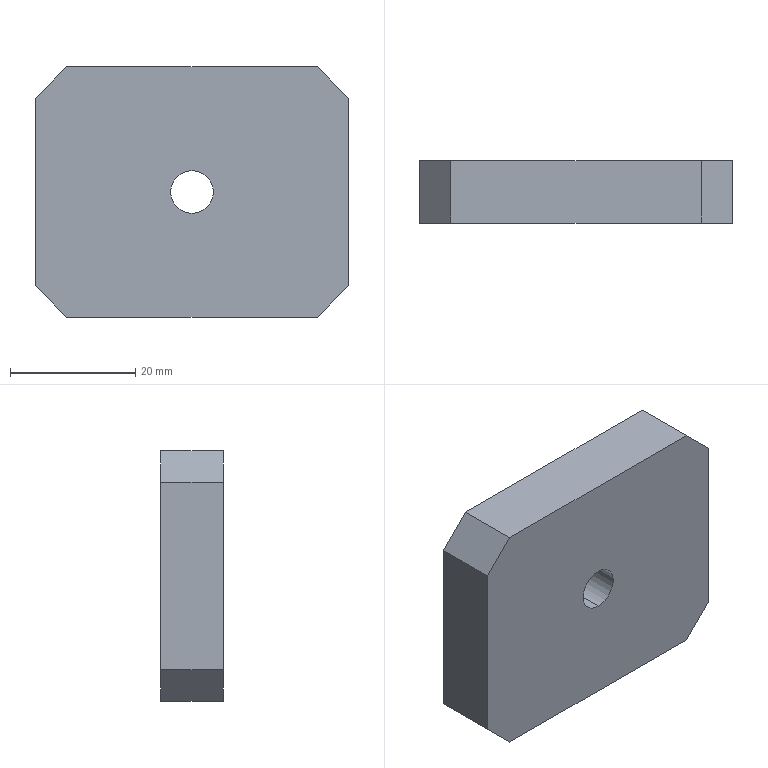Part | STEP file | 1 solid | 12 faces | box 50 x 10 x 40 mm | volume 19137 mm3 | plane 10 | cylinder 2 | commonest cylinder face diameters 6.8 x2
STEP:
#1=CARTESIAN_POINT('',(0.,0.,0.));
#2=DIRECTION('',(0.,0.,1.));
#3=DIRECTION('',(1.,0.,0.));
#4=AXIS2_PLACEMENT_3D('',#1,#2,#3);
#5=CARTESIAN_POINT('',(0.,0.,3.4));
#6=VERTEX_POINT('',#5);
#7=CARTESIAN_POINT('',(0.,10.,3.4));
#8=VERTEX_POINT('',#7);
#9=CARTESIAN_POINT('',(0.,0.,3.4));
#10=DIRECTION('',(0.,1.,0.));
#11=VECTOR('',#10,1.);
#12=LINE('',#9,#11);
#13=CARTESIAN_POINT('',(0.,0.,0.));
#14=DIRECTION('',(0.,1.,0.));
#15=DIRECTION('',(0.,0.,1.));
#16=AXIS2_PLACEMENT_3D('',#13,#14,#15);
#17=CYLINDRICAL_SURFACE('',#16,3.4);
#18=CARTESIAN_POINT('',(6.283,0.));
#19=DIRECTION('',(0.,1.));
#20=VECTOR('',#19,1.);
#21=LINE('',#18,#20);
#22=(GEOMETRIC_REPRESENTATION_CONTEXT(2)PARAMETRIC_REPRESENTATION_CONTEXT()REPRESENTATION_CONTEXT('',''));
#23=DEFINITIONAL_REPRESENTATION('',(#21),#22);
#24=PCURVE('',#17,#23);
#25=CARTESIAN_POINT('',(0.,0.,0.));
#26=DIRECTION('',(0.,1.,0.));
#27=DIRECTION('',(0.,0.,1.));
#28=AXIS2_PLACEMENT_3D('',#25,#26,#27);
#29=CYLINDRICAL_SURFACE('',#28,3.4);
#30=CARTESIAN_POINT('',(0.,0.));
#31=DIRECTION('',(0.,1.));
#32=VECTOR('',#31,1.);
#33=LINE('',#30,#32);
#34=(GEOMETRIC_REPRESENTATION_CONTEXT(2)PARAMETRIC_REPRESENTATION_CONTEXT()REPRESENTATION_CONTEXT('',''));
#35=DEFINITIONAL_REPRESENTATION('',(#33),#34);
#36=PCURVE('',#29,#35);
#37=SURFACE_CURVE('',#12,(#24,#36),.PCURVE_S1.);
#38=EDGE_CURVE('',#6,#8,#37,.T.);
#39=ORIENTED_EDGE('',*,*,#38,.T.);
#40=CARTESIAN_POINT('',(0.,10.,-3.4));
#41=VERTEX_POINT('',#40);
#42=CARTESIAN_POINT('',(0.,10.,0.));
#43=DIRECTION('',(0.,1.,0.));
#44=DIRECTION('',(0.,0.,1.));
#45=AXIS2_PLACEMENT_3D('',#42,#43,#44);
#46=CIRCLE('',#45,3.4);
#47=CARTESIAN_POINT('',(0.,10.));
#48=DIRECTION('',(1.,0.));
#49=VECTOR('',#48,1.);
#50=LINE('',#47,#49);
#51=(GEOMETRIC_REPRESENTATION_CONTEXT(2)PARAMETRIC_REPRESENTATION_CONTEXT()REPRESENTATION_CONTEXT('',''));
#52=DEFINITIONAL_REPRESENTATION('',(#50),#51);
#53=PCURVE('',#17,#52);
#54=CARTESIAN_POINT('',(-25.,10.,20.));
#55=DIRECTION('',(0.,-1.,0.));
#56=DIRECTION('',(0.,0.,-1.));
#57=AXIS2_PLACEMENT_3D('',#54,#55,#56);
#58=PLANE('',#57);
#59=CARTESIAN_POINT('',(16.6,25.));
#60=CARTESIAN_POINT('',(16.6,30.889));
#61=CARTESIAN_POINT('',(21.7,27.944));
#62=CARTESIAN_POINT('',(26.8,25.));
#63=CARTESIAN_POINT('',(21.7,22.056));
#64=CARTESIAN_POINT('',(16.6,19.111));
#65=CARTESIAN_POINT('',(16.6,25.));
#66=(BOUNDED_CURVE()B_SPLINE_CURVE(2,(#59,#60,#61,#62,#63,#64,#65),.UNSPECIFIED.,.T.,.F.)B_SPLINE_CURVE_WITH_KNOTS((1,2,2,2,2,1),(-2.094,0.,2.094,4.189,6.283,8.378),.UNSPECIFIED.)CURVE()GEOMETRIC_REPRESENTATION_ITEM()RATIONAL_B_SPLINE_CURVE((1.,0.5,1.,0.5,1.,0.5,1.))REPRESENTATION_ITEM(''));
#67=(GEOMETRIC_REPRESENTATION_CONTEXT(2)PARAMETRIC_REPRESENTATION_CONTEXT()REPRESENTATION_CONTEXT('',''));
#68=DEFINITIONAL_REPRESENTATION('',(#66),#67);
#69=PCURVE('',#58,#68);
#70=SURFACE_CURVE('',#46,(#53,#69),.PCURVE_S1.);
#71=EDGE_CURVE('',#41,#8,#70,.T.);
#72=ORIENTED_EDGE('',*,*,#71,.F.);
#73=CARTESIAN_POINT('',(0.,0.,-3.4));
#74=VERTEX_POINT('',#73);
#75=CARTESIAN_POINT('',(0.,0.,-3.4));
#76=DIRECTION('',(0.,1.,0.));
#77=VECTOR('',#76,1.);
#78=LINE('',#75,#77);
#79=CARTESIAN_POINT('',(3.142,0.));
#80=DIRECTION('',(0.,1.));
#81=VECTOR('',#80,1.);
#82=LINE('',#79,#81);
#83=(GEOMETRIC_REPRESENTATION_CONTEXT(2)PARAMETRIC_REPRESENTATION_CONTEXT()REPRESENTATION_CONTEXT('',''));
#84=DEFINITIONAL_REPRESENTATION('',(#82),#83);
#85=PCURVE('',#17,#84);
#86=CARTESIAN_POINT('',(3.142,0.));
#87=DIRECTION('',(0.,1.));
#88=VECTOR('',#87,1.);
#89=LINE('',#86,#88);
#90=(GEOMETRIC_REPRESENTATION_CONTEXT(2)PARAMETRIC_REPRESENTATION_CONTEXT()REPRESENTATION_CONTEXT('',''));
#91=DEFINITIONAL_REPRESENTATION('',(#89),#90);
#92=PCURVE('',#29,#91);
#93=SURFACE_CURVE('',#78,(#85,#92),.PCURVE_S1.);
#94=EDGE_CURVE('',#74,#41,#93,.T.);
#95=ORIENTED_EDGE('',*,*,#94,.F.);
#96=CARTESIAN_POINT('',(0.,0.,0.));
#97=DIRECTION('',(0.,-1.,0.));
#98=DIRECTION('',(0.,0.,1.));
#99=AXIS2_PLACEMENT_3D('',#96,#97,#98);
#100=CIRCLE('',#99,3.4);
#101=CARTESIAN_POINT('',(6.283,0.));
#102=DIRECTION('',(-1.,0.));
#103=VECTOR('',#102,1.);
#104=LINE('',#101,#103);
#105=(GEOMETRIC_REPRESENTATION_CONTEXT(2)PARAMETRIC_REPRESENTATION_CONTEXT()REPRESENTATION_CONTEXT('',''));
#106=DEFINITIONAL_REPRESENTATION('',(#104),#105);
#107=PCURVE('',#17,#106);
#108=CARTESIAN_POINT('',(-25.,0.,20.));
#109=DIRECTION('',(0.,-1.,0.));
#110=DIRECTION('',(0.,0.,-1.));
#111=AXIS2_PLACEMENT_3D('',#108,#109,#110);
#112=PLANE('',#111);
#113=CARTESIAN_POINT('',(20.,25.));
#114=DIRECTION('',(-1.,0.));
#115=AXIS2_PLACEMENT_2D('',#113,#114);
#116=CIRCLE('',#115,3.4);
#117=(GEOMETRIC_REPRESENTATION_CONTEXT(2)PARAMETRIC_REPRESENTATION_CONTEXT()REPRESENTATION_CONTEXT('',''));
#118=DEFINITIONAL_REPRESENTATION('',(#116),#117);
#119=PCURVE('',#112,#118);
#120=SURFACE_CURVE('',#100,(#107,#119),.PCURVE_S1.);
#121=EDGE_CURVE('',#6,#74,#120,.T.);
#122=ORIENTED_EDGE('',*,*,#121,.F.);
#123=EDGE_LOOP('',(#39,#72,#95,#122));
#124=FACE_BOUND('',#123,.F.);
#125=ADVANCED_FACE('',(#124),#17,.F.);
#126=CARTESIAN_POINT('',(0.,10.,0.));
#127=DIRECTION('',(0.,1.,0.));
#128=DIRECTION('',(0.,0.,1.));
#129=AXIS2_PLACEMENT_3D('',#126,#127,#128);
#130=CIRCLE('',#129,3.4);
#131=CARTESIAN_POINT('',(0.,10.));
#132=DIRECTION('',(1.,0.));
#133=VECTOR('',#132,1.);
#134=LINE('',#131,#133);
#135=(GEOMETRIC_REPRESENTATION_CONTEXT(2)PARAMETRIC_REPRESENTATION_CONTEXT()REPRESENTATION_CONTEXT('',''));
#136=DEFINITIONAL_REPRESENTATION('',(#134),#135);
#137=PCURVE('',#29,#136);
#138=CARTESIAN_POINT('',(16.6,25.));
#139=CARTESIAN_POINT('',(16.6,30.889));
#140=CARTESIAN_POINT('',(21.7,27.944));
#141=CARTESIAN_POINT('',(26.8,25.));
#142=CARTESIAN_POINT('',(21.7,22.056));
#143=CARTESIAN_POINT('',(16.6,19.111));
#144=CARTESIAN_POINT('',(16.6,25.));
#145=(BOUNDED_CURVE()B_SPLINE_CURVE(2,(#138,#139,#140,#141,#142,#143,#144),.UNSPECIFIED.,.T.,.F.)B_SPLINE_CURVE_WITH_KNOTS((1,2,2,2,2,1),(-2.094,0.,2.094,4.189,6.283,8.378),.UNSPECIFIED.)CURVE()GEOMETRIC_REPRESENTATION_ITEM()RATIONAL_B_SPLINE_CURVE((1.,0.5,1.,0.5,1.,0.5,1.))REPRESENTATION_ITEM(''));
#146=(GEOMETRIC_REPRESENTATION_CONTEXT(2)PARAMETRIC_REPRESENTATION_CONTEXT()REPRESENTATION_CONTEXT('',''));
#147=DEFINITIONAL_REPRESENTATION('',(#145),#146);
#148=PCURVE('',#58,#147);
#149=SURFACE_CURVE('',#130,(#137,#148),.PCURVE_S1.);
#150=EDGE_CURVE('',#8,#41,#149,.T.);
#151=ORIENTED_EDGE('',*,*,#150,.F.);
#152=ORIENTED_EDGE('',*,*,#38,.F.);
#153=CARTESIAN_POINT('',(0.,0.,0.));
#154=DIRECTION('',(0.,-1.,0.));
#155=DIRECTION('',(0.,0.,1.));
#156=AXIS2_PLACEMENT_3D('',#153,#154,#155);
#157=CIRCLE('',#156,3.4);
#158=CARTESIAN_POINT('',(6.283,0.));
#159=DIRECTION('',(-1.,0.));
#160=VECTOR('',#159,1.);
#161=LINE('',#158,#160);
#162=(GEOMETRIC_REPRESENTATION_CONTEXT(2)PARAMETRIC_REPRESENTATION_CONTEXT()REPRESENTATION_CONTEXT('',''));
#163=DEFINITIONAL_REPRESENTATION('',(#161),#162);
#164=PCURVE('',#29,#163);
#165=CARTESIAN_POINT('',(20.,25.));
#166=DIRECTION('',(-1.,0.));
#167=AXIS2_PLACEMENT_2D('',#165,#166);
#168=CIRCLE('',#167,3.4);
#169=(GEOMETRIC_REPRESENTATION_CONTEXT(2)PARAMETRIC_REPRESENTATION_CONTEXT()REPRESENTATION_CONTEXT('',''));
#170=DEFINITIONAL_REPRESENTATION('',(#168),#169);
#171=PCURVE('',#112,#170);
#172=SURFACE_CURVE('',#157,(#164,#171),.PCURVE_S1.);
#173=EDGE_CURVE('',#74,#6,#172,.T.);
#174=ORIENTED_EDGE('',*,*,#173,.F.);
#175=ORIENTED_EDGE('',*,*,#94,.T.);
#176=EDGE_LOOP('',(#151,#152,#174,#175));
#177=FACE_BOUND('',#176,.F.);
#178=ADVANCED_FACE('',(#177),#29,.F.);
#179=ORIENTED_EDGE('',*,*,#150,.F.);
#180=ORIENTED_EDGE('',*,*,#71,.F.);
#181=EDGE_LOOP('',(#179,#180));
#182=FACE_BOUND('',#181,.T.);
#183=CARTESIAN_POINT('',(-20.,10.,20.));
#184=VERTEX_POINT('',#183);
#185=CARTESIAN_POINT('',(-25.,10.,15.));
#186=VERTEX_POINT('',#185);
#187=CARTESIAN_POINT('',(-20.,10.,20.));
#188=DIRECTION('',(-0.7071,0.,-0.7071));
#189=VECTOR('',#188,1.);
#190=LINE('',#187,#189);
#191=CARTESIAN_POINT('',(0.,5.));
#192=DIRECTION('',(0.7071,-0.7071));
#193=VECTOR('',#192,1.);
#194=LINE('',#191,#193);
#195=(GEOMETRIC_REPRESENTATION_CONTEXT(2)PARAMETRIC_REPRESENTATION_CONTEXT()REPRESENTATION_CONTEXT('',''));
#196=DEFINITIONAL_REPRESENTATION('',(#194),#195);
#197=PCURVE('',#58,#196);
#198=CARTESIAN_POINT('',(-20.,10.,20.));
#199=DIRECTION('',(0.7071,0.,-0.7071));
#200=DIRECTION('',(0.,-1.,0.));
#201=AXIS2_PLACEMENT_3D('',#198,#199,#200);
#202=PLANE('',#201);
#203=CARTESIAN_POINT('',(0.,0.));
#204=DIRECTION('',(0.,1.));
#205=VECTOR('',#204,1.);
#206=LINE('',#203,#205);
#207=(GEOMETRIC_REPRESENTATION_CONTEXT(2)PARAMETRIC_REPRESENTATION_CONTEXT()REPRESENTATION_CONTEXT('',''));
#208=DEFINITIONAL_REPRESENTATION('',(#206),#207);
#209=PCURVE('',#202,#208);
#210=SURFACE_CURVE('',#190,(#197,#209),.PCURVE_S1.);
#211=EDGE_CURVE('',#184,#186,#210,.T.);
#212=ORIENTED_EDGE('',*,*,#211,.F.);
#213=CARTESIAN_POINT('',(20.,10.,20.));
#214=VERTEX_POINT('',#213);
#215=CARTESIAN_POINT('',(0.,10.,20.));
#216=DIRECTION('',(-1.,0.,0.));
#217=VECTOR('',#216,1.);
#218=LINE('',#215,#217);
#219=CARTESIAN_POINT('',(0.,25.));
#220=DIRECTION('',(0.,-1.));
#221=VECTOR('',#220,1.);
#222=LINE('',#219,#221);
#223=(GEOMETRIC_REPRESENTATION_CONTEXT(2)PARAMETRIC_REPRESENTATION_CONTEXT()REPRESENTATION_CONTEXT('',''));
#224=DEFINITIONAL_REPRESENTATION('',(#222),#223);
#225=PCURVE('',#58,#224);
#226=CARTESIAN_POINT('',(20.,0.,20.));
#227=DIRECTION('',(0.,0.,-1.));
#228=DIRECTION('',(-1.,0.,0.));
#229=AXIS2_PLACEMENT_3D('',#226,#227,#228);
#230=PLANE('',#229);
#231=CARTESIAN_POINT('',(20.,10.));
#232=DIRECTION('',(1.,0.));
#233=VECTOR('',#232,1.);
#234=LINE('',#231,#233);
#235=(GEOMETRIC_REPRESENTATION_CONTEXT(2)PARAMETRIC_REPRESENTATION_CONTEXT()REPRESENTATION_CONTEXT('',''));
#236=DEFINITIONAL_REPRESENTATION('',(#234),#235);
#237=PCURVE('',#230,#236);
#238=SURFACE_CURVE('',#218,(#225,#237),.PCURVE_S1.);
#239=EDGE_CURVE('',#214,#184,#238,.T.);
#240=ORIENTED_EDGE('',*,*,#239,.F.);
#241=CARTESIAN_POINT('',(25.,10.,15.));
#242=VERTEX_POINT('',#241);
#243=CARTESIAN_POINT('',(25.,10.,15.));
#244=DIRECTION('',(-0.7071,0.,0.7071));
#245=VECTOR('',#244,1.);
#246=LINE('',#243,#245);
#247=CARTESIAN_POINT('',(5.,50.));
#248=DIRECTION('',(-0.7071,-0.7071));
#249=VECTOR('',#248,1.);
#250=LINE('',#247,#249);
#251=(GEOMETRIC_REPRESENTATION_CONTEXT(2)PARAMETRIC_REPRESENTATION_CONTEXT()REPRESENTATION_CONTEXT('',''));
#252=DEFINITIONAL_REPRESENTATION('',(#250),#251);
#253=PCURVE('',#58,#252);
#254=CARTESIAN_POINT('',(25.,10.,15.));
#255=DIRECTION('',(-0.7071,0.,-0.7071));
#256=DIRECTION('',(0.,-1.,0.));
#257=AXIS2_PLACEMENT_3D('',#254,#255,#256);
#258=PLANE('',#257);
#259=CARTESIAN_POINT('',(0.,0.));
#260=DIRECTION('',(0.,1.));
#261=VECTOR('',#260,1.);
#262=LINE('',#259,#261);
#263=(GEOMETRIC_REPRESENTATION_CONTEXT(2)PARAMETRIC_REPRESENTATION_CONTEXT()REPRESENTATION_CONTEXT('',''));
#264=DEFINITIONAL_REPRESENTATION('',(#262),#263);
#265=PCURVE('',#258,#264);
#266=SURFACE_CURVE('',#246,(#253,#265),.PCURVE_S1.);
#267=EDGE_CURVE('',#242,#214,#266,.T.);
#268=ORIENTED_EDGE('',*,*,#267,.F.);
#269=CARTESIAN_POINT('',(25.,10.,-15.));
#270=VERTEX_POINT('',#269);
#271=CARTESIAN_POINT('',(25.,10.,0.));
#272=DIRECTION('',(0.,0.,1.));
#273=VECTOR('',#272,1.);
#274=LINE('',#271,#273);
#275=CARTESIAN_POINT('',(20.,50.));
#276=DIRECTION('',(-1.,0.));
#277=VECTOR('',#276,1.);
#278=LINE('',#275,#277);
#279=(GEOMETRIC_REPRESENTATION_CONTEXT(2)PARAMETRIC_REPRESENTATION_CONTEXT()REPRESENTATION_CONTEXT('',''));
#280=DEFINITIONAL_REPRESENTATION('',(#278),#279);
#281=PCURVE('',#58,#280);
#282=CARTESIAN_POINT('',(25.,0.,-15.));
#283=DIRECTION('',(-1.,0.,0.));
#284=DIRECTION('',(0.,0.,1.));
#285=AXIS2_PLACEMENT_3D('',#282,#283,#284);
#286=PLANE('',#285);
#287=CARTESIAN_POINT('',(15.,10.));
#288=DIRECTION('',(1.,0.));
#289=VECTOR('',#288,1.);
#290=LINE('',#287,#289);
#291=(GEOMETRIC_REPRESENTATION_CONTEXT(2)PARAMETRIC_REPRESENTATION_CONTEXT()REPRESENTATION_CONTEXT('',''));
#292=DEFINITIONAL_REPRESENTATION('',(#290),#291);
#293=PCURVE('',#286,#292);
#294=SURFACE_CURVE('',#274,(#281,#293),.PCURVE_S1.);
#295=EDGE_CURVE('',#270,#242,#294,.T.);
#296=ORIENTED_EDGE('',*,*,#295,.F.);
#297=CARTESIAN_POINT('',(20.,10.,-20.));
#298=VERTEX_POINT('',#297);
#299=CARTESIAN_POINT('',(20.,10.,-20.));
#300=DIRECTION('',(0.7071,0.,0.7071));
#301=VECTOR('',#300,1.);
#302=LINE('',#299,#301);
#303=CARTESIAN_POINT('',(40.,45.));
#304=DIRECTION('',(-0.7071,0.7071));
#305=VECTOR('',#304,1.);
#306=LINE('',#303,#305);
#307=(GEOMETRIC_REPRESENTATION_CONTEXT(2)PARAMETRIC_REPRESENTATION_CONTEXT()REPRESENTATION_CONTEXT('',''));
#308=DEFINITIONAL_REPRESENTATION('',(#306),#307);
#309=PCURVE('',#58,#308);
#310=CARTESIAN_POINT('',(20.,10.,-20.));
#311=DIRECTION('',(-0.7071,0.,0.7071));
#312=DIRECTION('',(0.,-1.,0.));
#313=AXIS2_PLACEMENT_3D('',#310,#311,#312);
#314=PLANE('',#313);
#315=CARTESIAN_POINT('',(0.,0.));
#316=DIRECTION('',(0.,1.));
#317=VECTOR('',#316,1.);
#318=LINE('',#315,#317);
#319=(GEOMETRIC_REPRESENTATION_CONTEXT(2)PARAMETRIC_REPRESENTATION_CONTEXT()REPRESENTATION_CONTEXT('',''));
#320=DEFINITIONAL_REPRESENTATION('',(#318),#319);
#321=PCURVE('',#314,#320);
#322=SURFACE_CURVE('',#302,(#309,#321),.PCURVE_S1.);
#323=EDGE_CURVE('',#298,#270,#322,.T.);
#324=ORIENTED_EDGE('',*,*,#323,.F.);
#325=CARTESIAN_POINT('',(-20.,10.,-20.));
#326=VERTEX_POINT('',#325);
#327=CARTESIAN_POINT('',(0.,10.,-20.));
#328=DIRECTION('',(1.,0.,0.));
#329=VECTOR('',#328,1.);
#330=LINE('',#327,#329);
#331=CARTESIAN_POINT('',(40.,25.));
#332=DIRECTION('',(0.,1.));
#333=VECTOR('',#332,1.);
#334=LINE('',#331,#333);
#335=(GEOMETRIC_REPRESENTATION_CONTEXT(2)PARAMETRIC_REPRESENTATION_CONTEXT()REPRESENTATION_CONTEXT('',''));
#336=DEFINITIONAL_REPRESENTATION('',(#334),#335);
#337=PCURVE('',#58,#336);
#338=CARTESIAN_POINT('',(-20.,0.,-20.));
#339=DIRECTION('',(0.,0.,1.));
#340=DIRECTION('',(1.,0.,0.));
#341=AXIS2_PLACEMENT_3D('',#338,#339,#340);
#342=PLANE('',#341);
#343=CARTESIAN_POINT('',(20.,10.));
#344=DIRECTION('',(1.,0.));
#345=VECTOR('',#344,1.);
#346=LINE('',#343,#345);
#347=(GEOMETRIC_REPRESENTATION_CONTEXT(2)PARAMETRIC_REPRESENTATION_CONTEXT()REPRESENTATION_CONTEXT('',''));
#348=DEFINITIONAL_REPRESENTATION('',(#346),#347);
#349=PCURVE('',#342,#348);
#350=SURFACE_CURVE('',#330,(#337,#349),.PCURVE_S1.);
#351=EDGE_CURVE('',#326,#298,#350,.T.);
#352=ORIENTED_EDGE('',*,*,#351,.F.);
#353=CARTESIAN_POINT('',(-25.,10.,-15.));
#354=VERTEX_POINT('',#353);
#355=CARTESIAN_POINT('',(-25.,10.,-15.));
#356=DIRECTION('',(0.7071,0.,-0.7071));
#357=VECTOR('',#356,1.);
#358=LINE('',#355,#357);
#359=CARTESIAN_POINT('',(35.,0.));
#360=DIRECTION('',(0.7071,0.7071));
#361=VECTOR('',#360,1.);
#362=LINE('',#359,#361);
#363=(GEOMETRIC_REPRESENTATION_CONTEXT(2)PARAMETRIC_REPRESENTATION_CONTEXT()REPRESENTATION_CONTEXT('',''));
#364=DEFINITIONAL_REPRESENTATION('',(#362),#363);
#365=PCURVE('',#58,#364);
#366=CARTESIAN_POINT('',(-25.,10.,-15.));
#367=DIRECTION('',(0.7071,0.,0.7071));
#368=DIRECTION('',(0.,-1.,0.));
#369=AXIS2_PLACEMENT_3D('',#366,#367,#368);
#370=PLANE('',#369);
#371=CARTESIAN_POINT('',(0.,0.));
#372=DIRECTION('',(0.,1.));
#373=VECTOR('',#372,1.);
#374=LINE('',#371,#373);
#375=(GEOMETRIC_REPRESENTATION_CONTEXT(2)PARAMETRIC_REPRESENTATION_CONTEXT()REPRESENTATION_CONTEXT('',''));
#376=DEFINITIONAL_REPRESENTATION('',(#374),#375);
#377=PCURVE('',#370,#376);
#378=SURFACE_CURVE('',#358,(#365,#377),.PCURVE_S1.);
#379=EDGE_CURVE('',#354,#326,#378,.T.);
#380=ORIENTED_EDGE('',*,*,#379,.F.);
#381=CARTESIAN_POINT('',(-25.,10.,0.));
#382=DIRECTION('',(0.,0.,-1.));
#383=VECTOR('',#382,1.);
#384=LINE('',#381,#383);
#385=CARTESIAN_POINT('',(20.,0.));
#386=DIRECTION('',(1.,0.));
#387=VECTOR('',#386,1.);
#388=LINE('',#385,#387);
#389=(GEOMETRIC_REPRESENTATION_CONTEXT(2)PARAMETRIC_REPRESENTATION_CONTEXT()REPRESENTATION_CONTEXT('',''));
#390=DEFINITIONAL_REPRESENTATION('',(#388),#389);
#391=PCURVE('',#58,#390);
#392=CARTESIAN_POINT('',(-25.,0.,15.));
#393=DIRECTION('',(1.,0.,0.));
#394=DIRECTION('',(0.,0.,-1.));
#395=AXIS2_PLACEMENT_3D('',#392,#393,#394);
#396=PLANE('',#395);
#397=CARTESIAN_POINT('',(15.,10.));
#398=DIRECTION('',(1.,0.));
#399=VECTOR('',#398,1.);
#400=LINE('',#397,#399);
#401=(GEOMETRIC_REPRESENTATION_CONTEXT(2)PARAMETRIC_REPRESENTATION_CONTEXT()REPRESENTATION_CONTEXT('',''));
#402=DEFINITIONAL_REPRESENTATION('',(#400),#401);
#403=PCURVE('',#396,#402);
#404=SURFACE_CURVE('',#384,(#391,#403),.PCURVE_S1.);
#405=EDGE_CURVE('',#186,#354,#404,.T.);
#406=ORIENTED_EDGE('',*,*,#405,.F.);
#407=EDGE_LOOP('',(#212,#240,#268,#296,#324,#352,#380,#406));
#408=FACE_BOUND('',#407,.T.);
#409=ADVANCED_FACE('',(#182,#408),#58,.F.);
#410=ORIENTED_EDGE('',*,*,#121,.F.);
#411=ORIENTED_EDGE('',*,*,#173,.F.);
#412=EDGE_LOOP('',(#410,#411));
#413=FACE_BOUND('',#412,.T.);
#414=CARTESIAN_POINT('',(25.,0.,-15.));
#415=VERTEX_POINT('',#414);
#416=CARTESIAN_POINT('',(25.,0.,15.));
#417=VERTEX_POINT('',#416);
#418=CARTESIAN_POINT('',(25.,0.,0.));
#419=DIRECTION('',(0.,0.,1.));
#420=VECTOR('',#419,1.);
#421=LINE('',#418,#420);
#422=CARTESIAN_POINT('',(20.,50.));
#423=DIRECTION('',(-1.,0.));
#424=VECTOR('',#423,1.);
#425=LINE('',#422,#424);
#426=(GEOMETRIC_REPRESENTATION_CONTEXT(2)PARAMETRIC_REPRESENTATION_CONTEXT()REPRESENTATION_CONTEXT('',''));
#427=DEFINITIONAL_REPRESENTATION('',(#425),#426);
#428=PCURVE('',#112,#427);
#429=CARTESIAN_POINT('',(15.,0.));
#430=DIRECTION('',(1.,0.));
#431=VECTOR('',#430,1.);
#432=LINE('',#429,#431);
#433=(GEOMETRIC_REPRESENTATION_CONTEXT(2)PARAMETRIC_REPRESENTATION_CONTEXT()REPRESENTATION_CONTEXT('',''));
#434=DEFINITIONAL_REPRESENTATION('',(#432),#433);
#435=PCURVE('',#286,#434);
#436=SURFACE_CURVE('',#421,(#428,#435),.PCURVE_S1.);
#437=EDGE_CURVE('',#415,#417,#436,.T.);
#438=ORIENTED_EDGE('',*,*,#437,.T.);
#439=CARTESIAN_POINT('',(20.,0.,20.));
#440=VERTEX_POINT('',#439);
#441=CARTESIAN_POINT('',(25.,0.,15.));
#442=DIRECTION('',(-0.7071,0.,0.7071));
#443=VECTOR('',#442,1.);
#444=LINE('',#441,#443);
#445=CARTESIAN_POINT('',(5.,50.));
#446=DIRECTION('',(-0.7071,-0.7071));
#447=VECTOR('',#446,1.);
#448=LINE('',#445,#447);
#449=(GEOMETRIC_REPRESENTATION_CONTEXT(2)PARAMETRIC_REPRESENTATION_CONTEXT()REPRESENTATION_CONTEXT('',''));
#450=DEFINITIONAL_REPRESENTATION('',(#448),#449);
#451=PCURVE('',#112,#450);
#452=CARTESIAN_POINT('',(10.,0.));
#453=DIRECTION('',(0.,1.));
#454=VECTOR('',#453,1.);
#455=LINE('',#452,#454);
#456=(GEOMETRIC_REPRESENTATION_CONTEXT(2)PARAMETRIC_REPRESENTATION_CONTEXT()REPRESENTATION_CONTEXT('',''));
#457=DEFINITIONAL_REPRESENTATION('',(#455),#456);
#458=PCURVE('',#258,#457);
#459=SURFACE_CURVE('',#444,(#451,#458),.PCURVE_S1.);
#460=EDGE_CURVE('',#417,#440,#459,.T.);
#461=ORIENTED_EDGE('',*,*,#460,.T.);
#462=CARTESIAN_POINT('',(-20.,0.,20.));
#463=VERTEX_POINT('',#462);
#464=CARTESIAN_POINT('',(0.,0.,20.));
#465=DIRECTION('',(-1.,0.,0.));
#466=VECTOR('',#465,1.);
#467=LINE('',#464,#466);
#468=CARTESIAN_POINT('',(0.,25.));
#469=DIRECTION('',(0.,-1.));
#470=VECTOR('',#469,1.);
#471=LINE('',#468,#470);
#472=(GEOMETRIC_REPRESENTATION_CONTEXT(2)PARAMETRIC_REPRESENTATION_CONTEXT()REPRESENTATION_CONTEXT('',''));
#473=DEFINITIONAL_REPRESENTATION('',(#471),#472);
#474=PCURVE('',#112,#473);
#475=CARTESIAN_POINT('',(20.,0.));
#476=DIRECTION('',(1.,0.));
#477=VECTOR('',#476,1.);
#478=LINE('',#475,#477);
#479=(GEOMETRIC_REPRESENTATION_CONTEXT(2)PARAMETRIC_REPRESENTATION_CONTEXT()REPRESENTATION_CONTEXT('',''));
#480=DEFINITIONAL_REPRESENTATION('',(#478),#479);
#481=PCURVE('',#230,#480);
#482=SURFACE_CURVE('',#467,(#474,#481),.PCURVE_S1.);
#483=EDGE_CURVE('',#440,#463,#482,.T.);
#484=ORIENTED_EDGE('',*,*,#483,.T.);
#485=CARTESIAN_POINT('',(-25.,0.,15.));
#486=VERTEX_POINT('',#485);
#487=CARTESIAN_POINT('',(-20.,0.,20.));
#488=DIRECTION('',(-0.7071,0.,-0.7071));
#489=VECTOR('',#488,1.);
#490=LINE('',#487,#489);
#491=CARTESIAN_POINT('',(0.,5.));
#492=DIRECTION('',(0.7071,-0.7071));
#493=VECTOR('',#492,1.);
#494=LINE('',#491,#493);
#495=(GEOMETRIC_REPRESENTATION_CONTEXT(2)PARAMETRIC_REPRESENTATION_CONTEXT()REPRESENTATION_CONTEXT('',''));
#496=DEFINITIONAL_REPRESENTATION('',(#494),#495);
#497=PCURVE('',#112,#496);
#498=CARTESIAN_POINT('',(10.,0.));
#499=DIRECTION('',(0.,1.));
#500=VECTOR('',#499,1.);
#501=LINE('',#498,#500);
#502=(GEOMETRIC_REPRESENTATION_CONTEXT(2)PARAMETRIC_REPRESENTATION_CONTEXT()REPRESENTATION_CONTEXT('',''));
#503=DEFINITIONAL_REPRESENTATION('',(#501),#502);
#504=PCURVE('',#202,#503);
#505=SURFACE_CURVE('',#490,(#497,#504),.PCURVE_S1.);
#506=EDGE_CURVE('',#463,#486,#505,.T.);
#507=ORIENTED_EDGE('',*,*,#506,.T.);
#508=CARTESIAN_POINT('',(-25.,0.,-15.));
#509=VERTEX_POINT('',#508);
#510=CARTESIAN_POINT('',(-25.,0.,0.));
#511=DIRECTION('',(0.,0.,-1.));
#512=VECTOR('',#511,1.);
#513=LINE('',#510,#512);
#514=CARTESIAN_POINT('',(20.,0.));
#515=DIRECTION('',(1.,0.));
#516=VECTOR('',#515,1.);
#517=LINE('',#514,#516);
#518=(GEOMETRIC_REPRESENTATION_CONTEXT(2)PARAMETRIC_REPRESENTATION_CONTEXT()REPRESENTATION_CONTEXT('',''));
#519=DEFINITIONAL_REPRESENTATION('',(#517),#518);
#520=PCURVE('',#112,#519);
#521=CARTESIAN_POINT('',(15.,0.));
#522=DIRECTION('',(1.,0.));
#523=VECTOR('',#522,1.);
#524=LINE('',#521,#523);
#525=(GEOMETRIC_REPRESENTATION_CONTEXT(2)PARAMETRIC_REPRESENTATION_CONTEXT()REPRESENTATION_CONTEXT('',''));
#526=DEFINITIONAL_REPRESENTATION('',(#524),#525);
#527=PCURVE('',#396,#526);
#528=SURFACE_CURVE('',#513,(#520,#527),.PCURVE_S1.);
#529=EDGE_CURVE('',#486,#509,#528,.T.);
#530=ORIENTED_EDGE('',*,*,#529,.T.);
#531=CARTESIAN_POINT('',(-20.,0.,-20.));
#532=VERTEX_POINT('',#531);
#533=CARTESIAN_POINT('',(-25.,0.,-15.));
#534=DIRECTION('',(0.7071,0.,-0.7071));
#535=VECTOR('',#534,1.);
#536=LINE('',#533,#535);
#537=CARTESIAN_POINT('',(35.,0.));
#538=DIRECTION('',(0.7071,0.7071));
#539=VECTOR('',#538,1.);
#540=LINE('',#537,#539);
#541=(GEOMETRIC_REPRESENTATION_CONTEXT(2)PARAMETRIC_REPRESENTATION_CONTEXT()REPRESENTATION_CONTEXT('',''));
#542=DEFINITIONAL_REPRESENTATION('',(#540),#541);
#543=PCURVE('',#112,#542);
#544=CARTESIAN_POINT('',(10.,0.));
#545=DIRECTION('',(0.,1.));
#546=VECTOR('',#545,1.);
#547=LINE('',#544,#546);
#548=(GEOMETRIC_REPRESENTATION_CONTEXT(2)PARAMETRIC_REPRESENTATION_CONTEXT()REPRESENTATION_CONTEXT('',''));
#549=DEFINITIONAL_REPRESENTATION('',(#547),#548);
#550=PCURVE('',#370,#549);
#551=SURFACE_CURVE('',#536,(#543,#550),.PCURVE_S1.);
#552=EDGE_CURVE('',#509,#532,#551,.T.);
#553=ORIENTED_EDGE('',*,*,#552,.T.);
#554=CARTESIAN_POINT('',(20.,0.,-20.));
#555=VERTEX_POINT('',#554);
#556=CARTESIAN_POINT('',(0.,0.,-20.));
#557=DIRECTION('',(1.,0.,0.));
#558=VECTOR('',#557,1.);
#559=LINE('',#556,#558);
#560=CARTESIAN_POINT('',(40.,25.));
#561=DIRECTION('',(0.,1.));
#562=VECTOR('',#561,1.);
#563=LINE('',#560,#562);
#564=(GEOMETRIC_REPRESENTATION_CONTEXT(2)PARAMETRIC_REPRESENTATION_CONTEXT()REPRESENTATION_CONTEXT('',''));
#565=DEFINITIONAL_REPRESENTATION('',(#563),#564);
#566=PCURVE('',#112,#565);
#567=CARTESIAN_POINT('',(20.,0.));
#568=DIRECTION('',(1.,0.));
#569=VECTOR('',#568,1.);
#570=LINE('',#567,#569);
#571=(GEOMETRIC_REPRESENTATION_CONTEXT(2)PARAMETRIC_REPRESENTATION_CONTEXT()REPRESENTATION_CONTEXT('',''));
#572=DEFINITIONAL_REPRESENTATION('',(#570),#571);
#573=PCURVE('',#342,#572);
#574=SURFACE_CURVE('',#559,(#566,#573),.PCURVE_S1.);
#575=EDGE_CURVE('',#532,#555,#574,.T.);
#576=ORIENTED_EDGE('',*,*,#575,.T.);
#577=CARTESIAN_POINT('',(20.,0.,-20.));
#578=DIRECTION('',(0.7071,0.,0.7071));
#579=VECTOR('',#578,1.);
#580=LINE('',#577,#579);
#581=CARTESIAN_POINT('',(40.,45.));
#582=DIRECTION('',(-0.7071,0.7071));
#583=VECTOR('',#582,1.);
#584=LINE('',#581,#583);
#585=(GEOMETRIC_REPRESENTATION_CONTEXT(2)PARAMETRIC_REPRESENTATION_CONTEXT()REPRESENTATION_CONTEXT('',''));
#586=DEFINITIONAL_REPRESENTATION('',(#584),#585);
#587=PCURVE('',#112,#586);
#588=CARTESIAN_POINT('',(10.,0.));
#589=DIRECTION('',(0.,1.));
#590=VECTOR('',#589,1.);
#591=LINE('',#588,#590);
#592=(GEOMETRIC_REPRESENTATION_CONTEXT(2)PARAMETRIC_REPRESENTATION_CONTEXT()REPRESENTATION_CONTEXT('',''));
#593=DEFINITIONAL_REPRESENTATION('',(#591),#592);
#594=PCURVE('',#314,#593);
#595=SURFACE_CURVE('',#580,(#587,#594),.PCURVE_S1.);
#596=EDGE_CURVE('',#555,#415,#595,.T.);
#597=ORIENTED_EDGE('',*,*,#596,.T.);
#598=EDGE_LOOP('',(#438,#461,#484,#507,#530,#553,#576,#597));
#599=FACE_BOUND('',#598,.T.);
#600=ADVANCED_FACE('',(#413,#599),#112,.T.);
#601=CARTESIAN_POINT('',(-25.,5.,15.));
#602=DIRECTION('',(0.,-1.,0.));
#603=VECTOR('',#602,1.);
#604=LINE('',#601,#603);
#605=CARTESIAN_POINT('',(0.,5.));
#606=DIRECTION('',(0.,-1.));
#607=VECTOR('',#606,1.);
#608=LINE('',#605,#607);
#609=(GEOMETRIC_REPRESENTATION_CONTEXT(2)PARAMETRIC_REPRESENTATION_CONTEXT()REPRESENTATION_CONTEXT('',''));
#610=DEFINITIONAL_REPRESENTATION('',(#608),#609);
#611=PCURVE('',#396,#610);
#612=CARTESIAN_POINT('',(5.,7.071));
#613=DIRECTION('',(1.,0.));
#614=VECTOR('',#613,1.);
#615=LINE('',#612,#614);
#616=(GEOMETRIC_REPRESENTATION_CONTEXT(2)PARAMETRIC_REPRESENTATION_CONTEXT()REPRESENTATION_CONTEXT('',''));
#617=DEFINITIONAL_REPRESENTATION('',(#615),#616);
#618=PCURVE('',#202,#617);
#619=SURFACE_CURVE('',#604,(#611,#618),.PCURVE_S1.);
#620=EDGE_CURVE('',#186,#486,#619,.T.);
#621=ORIENTED_EDGE('',*,*,#620,.F.);
#622=ORIENTED_EDGE('',*,*,#405,.T.);
#623=CARTESIAN_POINT('',(-25.,5.,-15.));
#624=DIRECTION('',(0.,1.,0.));
#625=VECTOR('',#624,1.);
#626=LINE('',#623,#625);
#627=CARTESIAN_POINT('',(30.,5.));
#628=DIRECTION('',(0.,1.));
#629=VECTOR('',#628,1.);
#630=LINE('',#627,#629);
#631=(GEOMETRIC_REPRESENTATION_CONTEXT(2)PARAMETRIC_REPRESENTATION_CONTEXT()REPRESENTATION_CONTEXT('',''));
#632=DEFINITIONAL_REPRESENTATION('',(#630),#631);
#633=PCURVE('',#396,#632);
#634=CARTESIAN_POINT('',(5.,0.));
#635=DIRECTION('',(-1.,0.));
#636=VECTOR('',#635,1.);
#637=LINE('',#634,#636);
#638=(GEOMETRIC_REPRESENTATION_CONTEXT(2)PARAMETRIC_REPRESENTATION_CONTEXT()REPRESENTATION_CONTEXT('',''));
#639=DEFINITIONAL_REPRESENTATION('',(#637),#638);
#640=PCURVE('',#370,#639);
#641=SURFACE_CURVE('',#626,(#633,#640),.PCURVE_S1.);
#642=EDGE_CURVE('',#509,#354,#641,.T.);
#643=ORIENTED_EDGE('',*,*,#642,.F.);
#644=ORIENTED_EDGE('',*,*,#529,.F.);
#645=EDGE_LOOP('',(#621,#622,#643,#644));
#646=FACE_BOUND('',#645,.T.);
#647=ADVANCED_FACE('',(#646),#396,.F.);
#648=ORIENTED_EDGE('',*,*,#620,.T.);
#649=ORIENTED_EDGE('',*,*,#506,.F.);
#650=CARTESIAN_POINT('',(-20.,5.,20.));
#651=DIRECTION('',(0.,-1.,0.));
#652=VECTOR('',#651,1.);
#653=LINE('',#650,#652);
#654=CARTESIAN_POINT('',(5.,0.));
#655=DIRECTION('',(1.,0.));
#656=VECTOR('',#655,1.);
#657=LINE('',#654,#656);
#658=(GEOMETRIC_REPRESENTATION_CONTEXT(2)PARAMETRIC_REPRESENTATION_CONTEXT()REPRESENTATION_CONTEXT('',''));
#659=DEFINITIONAL_REPRESENTATION('',(#657),#658);
#660=PCURVE('',#202,#659);
#661=CARTESIAN_POINT('',(40.,5.));
#662=DIRECTION('',(0.,-1.));
#663=VECTOR('',#662,1.);
#664=LINE('',#661,#663);
#665=(GEOMETRIC_REPRESENTATION_CONTEXT(2)PARAMETRIC_REPRESENTATION_CONTEXT()REPRESENTATION_CONTEXT('',''));
#666=DEFINITIONAL_REPRESENTATION('',(#664),#665);
#667=PCURVE('',#230,#666);
#668=SURFACE_CURVE('',#653,(#660,#667),.PCURVE_S1.);
#669=EDGE_CURVE('',#184,#463,#668,.T.);
#670=ORIENTED_EDGE('',*,*,#669,.F.);
#671=ORIENTED_EDGE('',*,*,#211,.T.);
#672=EDGE_LOOP('',(#648,#649,#670,#671));
#673=FACE_BOUND('',#672,.T.);
#674=ADVANCED_FACE('',(#673),#202,.F.);
#675=ORIENTED_EDGE('',*,*,#669,.T.);
#676=ORIENTED_EDGE('',*,*,#483,.F.);
#677=CARTESIAN_POINT('',(20.,5.,20.));
#678=DIRECTION('',(0.,-1.,0.));
#679=VECTOR('',#678,1.);
#680=LINE('',#677,#679);
#681=CARTESIAN_POINT('',(0.,5.));
#682=DIRECTION('',(0.,-1.));
#683=VECTOR('',#682,1.);
#684=LINE('',#681,#683);
#685=(GEOMETRIC_REPRESENTATION_CONTEXT(2)PARAMETRIC_REPRESENTATION_CONTEXT()REPRESENTATION_CONTEXT('',''));
#686=DEFINITIONAL_REPRESENTATION('',(#684),#685);
#687=PCURVE('',#230,#686);
#688=CARTESIAN_POINT('',(5.,7.071));
#689=DIRECTION('',(1.,0.));
#690=VECTOR('',#689,1.);
#691=LINE('',#688,#690);
#692=(GEOMETRIC_REPRESENTATION_CONTEXT(2)PARAMETRIC_REPRESENTATION_CONTEXT()REPRESENTATION_CONTEXT('',''));
#693=DEFINITIONAL_REPRESENTATION('',(#691),#692);
#694=PCURVE('',#258,#693);
#695=SURFACE_CURVE('',#680,(#687,#694),.PCURVE_S1.);
#696=EDGE_CURVE('',#214,#440,#695,.T.);
#697=ORIENTED_EDGE('',*,*,#696,.F.);
#698=ORIENTED_EDGE('',*,*,#239,.T.);
#699=EDGE_LOOP('',(#675,#676,#697,#698));
#700=FACE_BOUND('',#699,.T.);
#701=ADVANCED_FACE('',(#700),#230,.F.);
#702=ORIENTED_EDGE('',*,*,#696,.T.);
#703=ORIENTED_EDGE('',*,*,#460,.F.);
#704=CARTESIAN_POINT('',(25.,5.,15.));
#705=DIRECTION('',(0.,-1.,0.));
#706=VECTOR('',#705,1.);
#707=LINE('',#704,#706);
#708=CARTESIAN_POINT('',(5.,0.));
#709=DIRECTION('',(1.,0.));
#710=VECTOR('',#709,1.);
#711=LINE('',#708,#710);
#712=(GEOMETRIC_REPRESENTATION_CONTEXT(2)PARAMETRIC_REPRESENTATION_CONTEXT()REPRESENTATION_CONTEXT('',''));
#713=DEFINITIONAL_REPRESENTATION('',(#711),#712);
#714=PCURVE('',#258,#713);
#715=CARTESIAN_POINT('',(30.,5.));
#716=DIRECTION('',(0.,-1.));
#717=VECTOR('',#716,1.);
#718=LINE('',#715,#717);
#719=(GEOMETRIC_REPRESENTATION_CONTEXT(2)PARAMETRIC_REPRESENTATION_CONTEXT()REPRESENTATION_CONTEXT('',''));
#720=DEFINITIONAL_REPRESENTATION('',(#718),#719);
#721=PCURVE('',#286,#720);
#722=SURFACE_CURVE('',#707,(#714,#721),.PCURVE_S1.);
#723=EDGE_CURVE('',#242,#417,#722,.T.);
#724=ORIENTED_EDGE('',*,*,#723,.F.);
#725=ORIENTED_EDGE('',*,*,#267,.T.);
#726=EDGE_LOOP('',(#702,#703,#724,#725));
#727=FACE_BOUND('',#726,.T.);
#728=ADVANCED_FACE('',(#727),#258,.F.);
#729=CARTESIAN_POINT('',(25.,5.,-15.));
#730=DIRECTION('',(0.,-1.,0.));
#731=VECTOR('',#730,1.);
#732=LINE('',#729,#731);
#733=CARTESIAN_POINT('',(0.,5.));
#734=DIRECTION('',(0.,-1.));
#735=VECTOR('',#734,1.);
#736=LINE('',#733,#735);
#737=(GEOMETRIC_REPRESENTATION_CONTEXT(2)PARAMETRIC_REPRESENTATION_CONTEXT()REPRESENTATION_CONTEXT('',''));
#738=DEFINITIONAL_REPRESENTATION('',(#736),#737);
#739=PCURVE('',#286,#738);
#740=CARTESIAN_POINT('',(5.,7.071));
#741=DIRECTION('',(1.,0.));
#742=VECTOR('',#741,1.);
#743=LINE('',#740,#742);
#744=(GEOMETRIC_REPRESENTATION_CONTEXT(2)PARAMETRIC_REPRESENTATION_CONTEXT()REPRESENTATION_CONTEXT('',''));
#745=DEFINITIONAL_REPRESENTATION('',(#743),#744);
#746=PCURVE('',#314,#745);
#747=SURFACE_CURVE('',#732,(#739,#746),.PCURVE_S1.);
#748=EDGE_CURVE('',#270,#415,#747,.T.);
#749=ORIENTED_EDGE('',*,*,#748,.F.);
#750=ORIENTED_EDGE('',*,*,#295,.T.);
#751=ORIENTED_EDGE('',*,*,#723,.T.);
#752=ORIENTED_EDGE('',*,*,#437,.F.);
#753=EDGE_LOOP('',(#749,#750,#751,#752));
#754=FACE_BOUND('',#753,.T.);
#755=ADVANCED_FACE('',(#754),#286,.F.);
#756=ORIENTED_EDGE('',*,*,#748,.T.);
#757=ORIENTED_EDGE('',*,*,#596,.F.);
#758=CARTESIAN_POINT('',(20.,5.,-20.));
#759=DIRECTION('',(0.,-1.,0.));
#760=VECTOR('',#759,1.);
#761=LINE('',#758,#760);
#762=CARTESIAN_POINT('',(5.,0.));
#763=DIRECTION('',(1.,0.));
#764=VECTOR('',#763,1.);
#765=LINE('',#762,#764);
#766=(GEOMETRIC_REPRESENTATION_CONTEXT(2)PARAMETRIC_REPRESENTATION_CONTEXT()REPRESENTATION_CONTEXT('',''));
#767=DEFINITIONAL_REPRESENTATION('',(#765),#766);
#768=PCURVE('',#314,#767);
#769=CARTESIAN_POINT('',(40.,5.));
#770=DIRECTION('',(0.,-1.));
#771=VECTOR('',#770,1.);
#772=LINE('',#769,#771);
#773=(GEOMETRIC_REPRESENTATION_CONTEXT(2)PARAMETRIC_REPRESENTATION_CONTEXT()REPRESENTATION_CONTEXT('',''));
#774=DEFINITIONAL_REPRESENTATION('',(#772),#773);
#775=PCURVE('',#342,#774);
#776=SURFACE_CURVE('',#761,(#768,#775),.PCURVE_S1.);
#777=EDGE_CURVE('',#298,#555,#776,.T.);
#778=ORIENTED_EDGE('',*,*,#777,.F.);
#779=ORIENTED_EDGE('',*,*,#323,.T.);
#780=EDGE_LOOP('',(#756,#757,#778,#779));
#781=FACE_BOUND('',#780,.T.);
#782=ADVANCED_FACE('',(#781),#314,.F.);
#783=CARTESIAN_POINT('',(-20.,5.,-20.));
#784=DIRECTION('',(0.,-1.,0.));
#785=VECTOR('',#784,1.);
#786=LINE('',#783,#785);
#787=CARTESIAN_POINT('',(0.,5.));
#788=DIRECTION('',(0.,-1.));
#789=VECTOR('',#788,1.);
#790=LINE('',#787,#789);
#791=(GEOMETRIC_REPRESENTATION_CONTEXT(2)PARAMETRIC_REPRESENTATION_CONTEXT()REPRESENTATION_CONTEXT('',''));
#792=DEFINITIONAL_REPRESENTATION('',(#790),#791);
#793=PCURVE('',#342,#792);
#794=CARTESIAN_POINT('',(5.,7.071));
#795=DIRECTION('',(1.,0.));
#796=VECTOR('',#795,1.);
#797=LINE('',#794,#796);
#798=(GEOMETRIC_REPRESENTATION_CONTEXT(2)PARAMETRIC_REPRESENTATION_CONTEXT()REPRESENTATION_CONTEXT('',''));
#799=DEFINITIONAL_REPRESENTATION('',(#797),#798);
#800=PCURVE('',#370,#799);
#801=SURFACE_CURVE('',#786,(#793,#800),.PCURVE_S1.);
#802=EDGE_CURVE('',#326,#532,#801,.T.);
#803=ORIENTED_EDGE('',*,*,#802,.F.);
#804=ORIENTED_EDGE('',*,*,#351,.T.);
#805=ORIENTED_EDGE('',*,*,#777,.T.);
#806=ORIENTED_EDGE('',*,*,#575,.F.);
#807=EDGE_LOOP('',(#803,#804,#805,#806));
#808=FACE_BOUND('',#807,.T.);
#809=ADVANCED_FACE('',(#808),#342,.F.);
#810=ORIENTED_EDGE('',*,*,#802,.T.);
#811=ORIENTED_EDGE('',*,*,#552,.F.);
#812=ORIENTED_EDGE('',*,*,#642,.T.);
#813=ORIENTED_EDGE('',*,*,#379,.T.);
#814=EDGE_LOOP('',(#810,#811,#812,#813));
#815=FACE_BOUND('',#814,.T.);
#816=ADVANCED_FACE('',(#815),#370,.F.);
#817=CLOSED_SHELL('',(#125,#178,#409,#600,#647,#674,#701,#728,#755,#782,#809,#816));
#818=MANIFOLD_SOLID_BREP('',#817);
#819=(LENGTH_UNIT()NAMED_UNIT(*)SI_UNIT(.MILLI.,.METRE.));
#820=UNCERTAINTY_MEASURE_WITH_UNIT(LENGTH_MEASURE(0.0000001),#819,'','');
#821=(NAMED_UNIT(*)PLANE_ANGLE_UNIT()SI_UNIT($,.RADIAN.));
#822=(NAMED_UNIT(*)SI_UNIT($,.STERADIAN.)SOLID_ANGLE_UNIT());
#823=(GEOMETRIC_REPRESENTATION_CONTEXT(3)GLOBAL_UNCERTAINTY_ASSIGNED_CONTEXT((#820))GLOBAL_UNIT_ASSIGNED_CONTEXT((#819,#821,#822))REPRESENTATION_CONTEXT('',''));
#824=ADVANCED_BREP_SHAPE_REPRESENTATION('',(#4,#818),#823);